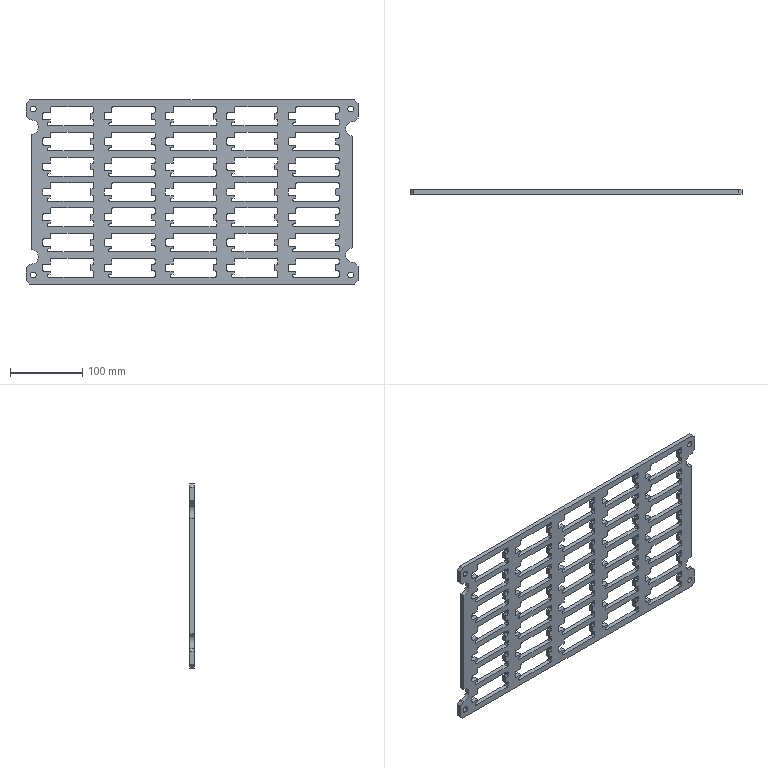Part | STEP file | X77-09211a | 1 solid | 945 faces | box 460.001 x 6 x 255 mm | volume 335353 mm3 | plane 512 | cylinder 433 | commonest cylinder face diameters 4 x349 1 x70 8 x8 20 x4 20.3 x2